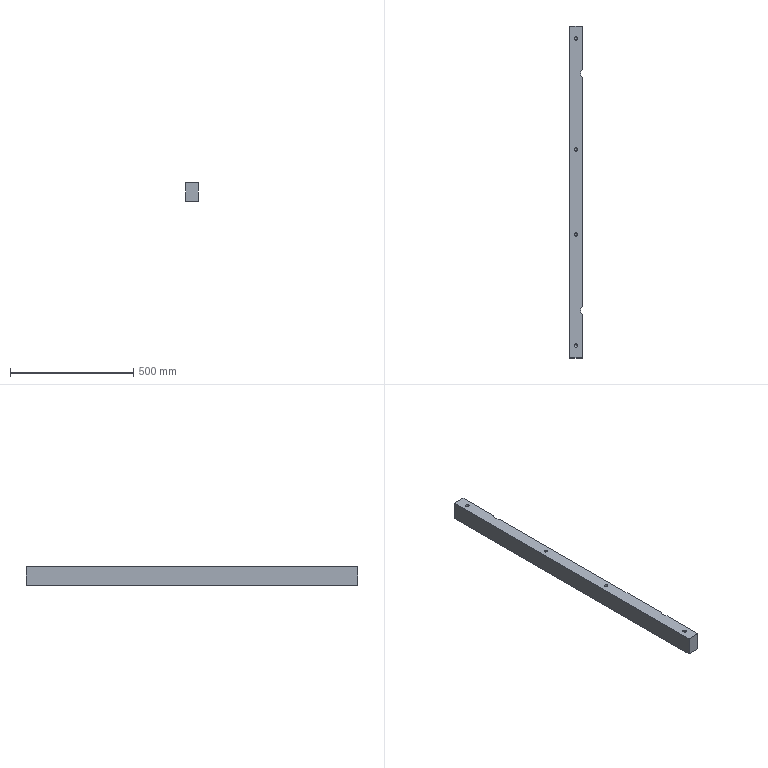Part | NX | features 3 2 | 1 solid | 26 faces | box 50 x 1345 x 75.5 mm | volume 5041133 mm3 | cylinder 10 | plane 8 | cone 8 | commonest cylinder face diameters 14.1 x8 53 x2
STEP:
#1=CARTESIAN_POINT('',(3352.05,-622.5,256.5));
#2=VERTEX_POINT('',#1);
#3=CARTESIAN_POINT('',(3345.,-622.5,256.5));
#4=DIRECTION('',(0.,0.,-1.));
#5=DIRECTION('',(1.,0.,0.));
#6=AXIS2_PLACEMENT_3D('',#3,#4,#5);
#7=CIRCLE('',#6,7.05);
#8=EDGE_CURVE('',#2,#2,#7,.T.);
#9=ORIENTED_EDGE('',*,*,#8,.T.);
#10=EDGE_LOOP('',(#9));
#11=FACE_BOUND('',#10,.T.);
#12=CARTESIAN_POINT('',(3352.05,622.5,256.5));
#13=VERTEX_POINT('',#12);
#14=CARTESIAN_POINT('',(3345.,622.5,256.5));
#15=DIRECTION('',(0.,0.,-1.));
#16=DIRECTION('',(1.,0.,0.));
#17=AXIS2_PLACEMENT_3D('',#14,#15,#16);
#18=CIRCLE('',#17,7.05);
#19=EDGE_CURVE('',#13,#13,#18,.T.);
#20=ORIENTED_EDGE('',*,*,#19,.T.);
#21=EDGE_LOOP('',(#20));
#22=FACE_BOUND('',#21,.T.);
#23=CARTESIAN_POINT('',(3370.,-497.385,256.5));
#24=VERTEX_POINT('',#23);
#25=CARTESIAN_POINT('',(3370.,-462.615,256.5));
#26=VERTEX_POINT('',#25);
#27=CARTESIAN_POINT('',(3390.,-480.,256.5));
#28=DIRECTION('',(0.,0.,-1.));
#29=DIRECTION('',(1.,0.,0.));
#30=AXIS2_PLACEMENT_3D('',#27,#28,#29);
#31=CIRCLE('',#30,26.5);
#32=EDGE_CURVE('',#24,#26,#31,.T.);
#33=ORIENTED_EDGE('',*,*,#32,.T.);
#34=CARTESIAN_POINT('',(3370.,462.615,256.5));
#35=VERTEX_POINT('',#34);
#36=CARTESIAN_POINT('',(3370.,193.,256.5));
#37=DIRECTION('',(0.,1.,0.));
#38=VECTOR('',#37,1000.);
#39=LINE('',#36,#38);
#40=EDGE_CURVE('',#26,#35,#39,.T.);
#41=ORIENTED_EDGE('',*,*,#40,.T.);
#42=CARTESIAN_POINT('',(3370.,497.385,256.5));
#43=VERTEX_POINT('',#42);
#44=CARTESIAN_POINT('',(3390.,480.,256.5));
#45=DIRECTION('',(0.,0.,1.));
#46=DIRECTION('',(1.,0.,0.));
#47=AXIS2_PLACEMENT_3D('',#44,#45,#46);
#48=CIRCLE('',#47,26.5);
#49=EDGE_CURVE('',#43,#35,#48,.T.);
#50=ORIENTED_EDGE('',*,*,#49,.F.);
#51=CARTESIAN_POINT('',(3370.,672.5,256.5));
#52=VERTEX_POINT('',#51);
#53=CARTESIAN_POINT('',(3370.,193.,256.5));
#54=DIRECTION('',(0.,1.,0.));
#55=VECTOR('',#54,1000.);
#56=LINE('',#53,#55);
#57=EDGE_CURVE('',#43,#52,#56,.T.);
#58=ORIENTED_EDGE('',*,*,#57,.T.);
#59=CARTESIAN_POINT('',(3320.,672.5,256.5));
#60=VERTEX_POINT('',#59);
#61=CARTESIAN_POINT('',(1330.,672.5,256.5));
#62=DIRECTION('',(-1.,0.,0.));
#63=VECTOR('',#62,1000.);
#64=LINE('',#61,#63);
#65=EDGE_CURVE('',#52,#60,#64,.T.);
#66=ORIENTED_EDGE('',*,*,#65,.T.);
#67=CARTESIAN_POINT('',(3320.,-672.5,256.5));
#68=VERTEX_POINT('',#67);
#69=CARTESIAN_POINT('',(3320.,193.,256.5));
#70=DIRECTION('',(0.,-1.,0.));
#71=VECTOR('',#70,1000.);
#72=LINE('',#69,#71);
#73=EDGE_CURVE('',#60,#68,#72,.T.);
#74=ORIENTED_EDGE('',*,*,#73,.T.);
#75=CARTESIAN_POINT('',(3370.,-672.5,256.5));
#76=VERTEX_POINT('',#75);
#77=CARTESIAN_POINT('',(1330.,-672.5,256.5));
#78=DIRECTION('',(1.,0.,0.));
#79=VECTOR('',#78,1000.);
#80=LINE('',#77,#79);
#81=EDGE_CURVE('',#68,#76,#80,.T.);
#82=ORIENTED_EDGE('',*,*,#81,.T.);
#83=CARTESIAN_POINT('',(3370.,193.,256.5));
#84=DIRECTION('',(0.,1.,0.));
#85=VECTOR('',#84,1000.);
#86=LINE('',#83,#85);
#87=EDGE_CURVE('',#76,#24,#86,.T.);
#88=ORIENTED_EDGE('',*,*,#87,.T.);
#89=EDGE_LOOP('',(#33,#41,#50,#58,#66,#74,#82,#88));
#90=FACE_BOUND('',#89,.T.);
#91=CARTESIAN_POINT('',(3352.05,172.5,256.5));
#92=VERTEX_POINT('',#91);
#93=CARTESIAN_POINT('',(3345.,172.5,256.5));
#94=DIRECTION('',(0.,0.,-1.));
#95=DIRECTION('',(1.,0.,0.));
#96=AXIS2_PLACEMENT_3D('',#93,#94,#95);
#97=CIRCLE('',#96,7.05);
#98=EDGE_CURVE('',#92,#92,#97,.T.);
#99=ORIENTED_EDGE('',*,*,#98,.T.);
#100=EDGE_LOOP('',(#99));
#101=FACE_BOUND('',#100,.T.);
#102=CARTESIAN_POINT('',(3352.05,-172.5,256.5));
#103=VERTEX_POINT('',#102);
#104=CARTESIAN_POINT('',(3345.,-172.5,256.5));
#105=DIRECTION('',(0.,0.,-1.));
#106=DIRECTION('',(1.,0.,0.));
#107=AXIS2_PLACEMENT_3D('',#104,#105,#106);
#108=CIRCLE('',#107,7.05);
#109=EDGE_CURVE('',#103,#103,#108,.T.);
#110=ORIENTED_EDGE('',*,*,#109,.T.);
#111=EDGE_LOOP('',(#110));
#112=FACE_BOUND('',#111,.T.);
#113=CARTESIAN_POINT('',(1330.,0.,256.5));
#114=DIRECTION('',(0.,0.,1.));
#115=DIRECTION('',(1.,0.,0.));
#116=AXIS2_PLACEMENT_3D('',#113,#114,#115);
#117=PLANE('',#116);
#118=ADVANCED_FACE('',(#11,#22,#90,#101,#112),#117,.T.);
#119=CARTESIAN_POINT('',(3352.05,-172.5,181.));
#120=VERTEX_POINT('',#119);
#121=CARTESIAN_POINT('',(3345.,-172.5,181.));
#122=DIRECTION('',(0.,0.,1.));
#123=DIRECTION('',(1.,0.,0.));
#124=AXIS2_PLACEMENT_3D('',#121,#122,#123);
#125=CIRCLE('',#124,7.05);
#126=EDGE_CURVE('',#120,#120,#125,.T.);
#127=ORIENTED_EDGE('',*,*,#126,.T.);
#128=EDGE_LOOP('',(#127));
#129=FACE_BOUND('',#128,.T.);
#130=CARTESIAN_POINT('',(3352.05,172.5,181.));
#131=VERTEX_POINT('',#130);
#132=CARTESIAN_POINT('',(3345.,172.5,181.));
#133=DIRECTION('',(0.,0.,1.));
#134=DIRECTION('',(1.,0.,0.));
#135=AXIS2_PLACEMENT_3D('',#132,#133,#134);
#136=CIRCLE('',#135,7.05);
#137=EDGE_CURVE('',#131,#131,#136,.T.);
#138=ORIENTED_EDGE('',*,*,#137,.T.);
#139=EDGE_LOOP('',(#138));
#140=FACE_BOUND('',#139,.T.);
#141=CARTESIAN_POINT('',(3370.,-497.385,181.));
#142=VERTEX_POINT('',#141);
#143=CARTESIAN_POINT('',(3370.,-462.615,181.));
#144=VERTEX_POINT('',#143);
#145=CARTESIAN_POINT('',(3390.,-480.,181.));
#146=DIRECTION('',(0.,0.,-1.));
#147=DIRECTION('',(-1.,0.,0.));
#148=AXIS2_PLACEMENT_3D('',#145,#146,#147);
#149=CIRCLE('',#148,26.5);
#150=EDGE_CURVE('',#142,#144,#149,.T.);
#151=ORIENTED_EDGE('',*,*,#150,.F.);
#152=CARTESIAN_POINT('',(3370.,-672.5,181.));
#153=VERTEX_POINT('',#152);
#154=CARTESIAN_POINT('',(3370.,193.,181.));
#155=DIRECTION('',(0.,-1.,0.));
#156=VECTOR('',#155,1000.);
#157=LINE('',#154,#156);
#158=EDGE_CURVE('',#142,#153,#157,.T.);
#159=ORIENTED_EDGE('',*,*,#158,.T.);
#160=CARTESIAN_POINT('',(3320.,-672.5,181.));
#161=VERTEX_POINT('',#160);
#162=CARTESIAN_POINT('',(267.5,-672.5,181.));
#163=DIRECTION('',(1.,0.,0.));
#164=VECTOR('',#163,1000.);
#165=LINE('',#162,#164);
#166=EDGE_CURVE('',#161,#153,#165,.T.);
#167=ORIENTED_EDGE('',*,*,#166,.F.);
#168=CARTESIAN_POINT('',(3320.,672.5,181.));
#169=VERTEX_POINT('',#168);
#170=CARTESIAN_POINT('',(3320.,193.,181.));
#171=DIRECTION('',(0.,1.,0.));
#172=VECTOR('',#171,1000.);
#173=LINE('',#170,#172);
#174=EDGE_CURVE('',#161,#169,#173,.T.);
#175=ORIENTED_EDGE('',*,*,#174,.T.);
#176=CARTESIAN_POINT('',(3370.,672.5,181.));
#177=VERTEX_POINT('',#176);
#178=CARTESIAN_POINT('',(3370.,672.5,181.));
#179=DIRECTION('',(-1.,0.,0.));
#180=VECTOR('',#179,1000.);
#181=LINE('',#178,#180);
#182=EDGE_CURVE('',#177,#169,#181,.T.);
#183=ORIENTED_EDGE('',*,*,#182,.F.);
#184=CARTESIAN_POINT('',(3370.,497.385,181.));
#185=VERTEX_POINT('',#184);
#186=CARTESIAN_POINT('',(3370.,193.,181.));
#187=DIRECTION('',(0.,-1.,0.));
#188=VECTOR('',#187,1000.);
#189=LINE('',#186,#188);
#190=EDGE_CURVE('',#177,#185,#189,.T.);
#191=ORIENTED_EDGE('',*,*,#190,.T.);
#192=CARTESIAN_POINT('',(3370.,462.615,181.));
#193=VERTEX_POINT('',#192);
#194=CARTESIAN_POINT('',(3390.,480.,181.));
#195=DIRECTION('',(0.,0.,1.));
#196=DIRECTION('',(-1.,0.,0.));
#197=AXIS2_PLACEMENT_3D('',#194,#195,#196);
#198=CIRCLE('',#197,26.5);
#199=EDGE_CURVE('',#185,#193,#198,.T.);
#200=ORIENTED_EDGE('',*,*,#199,.T.);
#201=CARTESIAN_POINT('',(3370.,193.,181.));
#202=DIRECTION('',(0.,-1.,0.));
#203=VECTOR('',#202,1000.);
#204=LINE('',#201,#203);
#205=EDGE_CURVE('',#193,#144,#204,.T.);
#206=ORIENTED_EDGE('',*,*,#205,.T.);
#207=EDGE_LOOP('',(#151,#159,#167,#175,#183,#191,#200,#206));
#208=FACE_BOUND('',#207,.T.);
#209=CARTESIAN_POINT('',(3352.05,-622.5,181.));
#210=VERTEX_POINT('',#209);
#211=CARTESIAN_POINT('',(3345.,-622.5,181.));
#212=DIRECTION('',(0.,0.,1.));
#213=DIRECTION('',(1.,0.,0.));
#214=AXIS2_PLACEMENT_3D('',#211,#212,#213);
#215=CIRCLE('',#214,7.05);
#216=EDGE_CURVE('',#210,#210,#215,.T.);
#217=ORIENTED_EDGE('',*,*,#216,.T.);
#218=EDGE_LOOP('',(#217));
#219=FACE_BOUND('',#218,.T.);
#220=CARTESIAN_POINT('',(3352.05,622.5,181.));
#221=VERTEX_POINT('',#220);
#222=CARTESIAN_POINT('',(3345.,622.5,181.));
#223=DIRECTION('',(0.,0.,1.));
#224=DIRECTION('',(1.,0.,0.));
#225=AXIS2_PLACEMENT_3D('',#222,#223,#224);
#226=CIRCLE('',#225,7.05);
#227=EDGE_CURVE('',#221,#221,#226,.T.);
#228=ORIENTED_EDGE('',*,*,#227,.T.);
#229=EDGE_LOOP('',(#228));
#230=FACE_BOUND('',#229,.T.);
#231=CARTESIAN_POINT('',(2100.,193.,181.));
#232=DIRECTION('',(0.,0.,-1.));
#233=DIRECTION('',(1.,0.,0.));
#234=AXIS2_PLACEMENT_3D('',#231,#232,#233);
#235=PLANE('',#234);
#236=ADVANCED_FACE('',(#129,#140,#208,#219,#230),#235,.T.);
#237=CARTESIAN_POINT('',(3370.,-462.615,181.));
#238=DIRECTION('',(0.,0.,1.));
#239=VECTOR('',#238,1000.);
#240=LINE('',#237,#239);
#241=EDGE_CURVE('',#144,#26,#240,.T.);
#242=ORIENTED_EDGE('',*,*,#241,.F.);
#243=ORIENTED_EDGE('',*,*,#205,.F.);
#244=CARTESIAN_POINT('',(3370.,462.615,181.));
#245=DIRECTION('',(0.,0.,1.));
#246=VECTOR('',#245,1000.);
#247=LINE('',#244,#246);
#248=EDGE_CURVE('',#193,#35,#247,.T.);
#249=ORIENTED_EDGE('',*,*,#248,.T.);
#250=ORIENTED_EDGE('',*,*,#40,.F.);
#251=EDGE_LOOP('',(#242,#243,#249,#250));
#252=FACE_BOUND('',#251,.T.);
#253=CARTESIAN_POINT('',(3370.,193.,-1.5));
#254=DIRECTION('',(1.,0.,0.));
#255=DIRECTION('',(0.,0.,-1.));
#256=AXIS2_PLACEMENT_3D('',#253,#254,#255);
#257=PLANE('',#256);
#258=ADVANCED_FACE('',(#252),#257,.T.);
#259=CARTESIAN_POINT('',(3370.,497.385,256.5));
#260=DIRECTION('',(0.,0.,-1.));
#261=VECTOR('',#260,1000.);
#262=LINE('',#259,#261);
#263=EDGE_CURVE('',#43,#185,#262,.T.);
#264=ORIENTED_EDGE('',*,*,#263,.T.);
#265=ORIENTED_EDGE('',*,*,#190,.F.);
#266=CARTESIAN_POINT('',(3370.,672.5,231.5));
#267=DIRECTION('',(0.,0.,-1.));
#268=VECTOR('',#267,1000.);
#269=LINE('',#266,#268);
#270=EDGE_CURVE('',#52,#177,#269,.T.);
#271=ORIENTED_EDGE('',*,*,#270,.F.);
#272=ORIENTED_EDGE('',*,*,#57,.F.);
#273=EDGE_LOOP('',(#264,#265,#271,#272));
#274=FACE_BOUND('',#273,.T.);
#275=CARTESIAN_POINT('',(3370.,193.,-1.5));
#276=DIRECTION('',(1.,0.,0.));
#277=DIRECTION('',(0.,0.,-1.));
#278=AXIS2_PLACEMENT_3D('',#275,#276,#277);
#279=PLANE('',#278);
#280=ADVANCED_FACE('',(#274),#279,.T.);
#281=CARTESIAN_POINT('',(3370.,-497.385,256.5));
#282=DIRECTION('',(0.,0.,-1.));
#283=VECTOR('',#282,1000.);
#284=LINE('',#281,#283);
#285=EDGE_CURVE('',#24,#142,#284,.T.);
#286=ORIENTED_EDGE('',*,*,#285,.F.);
#287=ORIENTED_EDGE('',*,*,#87,.F.);
#288=CARTESIAN_POINT('',(3370.,-672.5,-103.));
#289=DIRECTION('',(0.,0.,1.));
#290=VECTOR('',#289,1000.);
#291=LINE('',#288,#290);
#292=EDGE_CURVE('',#153,#76,#291,.T.);
#293=ORIENTED_EDGE('',*,*,#292,.F.);
#294=ORIENTED_EDGE('',*,*,#158,.F.);
#295=EDGE_LOOP('',(#286,#287,#293,#294));
#296=FACE_BOUND('',#295,.T.);
#297=CARTESIAN_POINT('',(3370.,193.,-1.5));
#298=DIRECTION('',(1.,0.,0.));
#299=DIRECTION('',(0.,0.,-1.));
#300=AXIS2_PLACEMENT_3D('',#297,#298,#299);
#301=PLANE('',#300);
#302=ADVANCED_FACE('',(#296),#301,.T.);
#303=CARTESIAN_POINT('',(3320.,672.5,231.5));
#304=DIRECTION('',(0.,0.,1.));
#305=VECTOR('',#304,1000.);
#306=LINE('',#303,#305);
#307=EDGE_CURVE('',#169,#60,#306,.T.);
#308=ORIENTED_EDGE('',*,*,#307,.F.);
#309=ORIENTED_EDGE('',*,*,#174,.F.);
#310=CARTESIAN_POINT('',(3320.,-672.5,-103.));
#311=DIRECTION('',(0.,0.,-1.));
#312=VECTOR('',#311,1000.);
#313=LINE('',#310,#312);
#314=EDGE_CURVE('',#68,#161,#313,.T.);
#315=ORIENTED_EDGE('',*,*,#314,.F.);
#316=ORIENTED_EDGE('',*,*,#73,.F.);
#317=EDGE_LOOP('',(#308,#309,#315,#316));
#318=FACE_BOUND('',#317,.T.);
#319=CARTESIAN_POINT('',(3320.,193.,-1.5));
#320=DIRECTION('',(-1.,0.,0.));
#321=DIRECTION('',(0.,0.,1.));
#322=AXIS2_PLACEMENT_3D('',#319,#320,#321);
#323=PLANE('',#322);
#324=ADVANCED_FACE('',(#318),#323,.T.);
#325=ORIENTED_EDGE('',*,*,#314,.T.);
#326=ORIENTED_EDGE('',*,*,#166,.T.);
#327=ORIENTED_EDGE('',*,*,#292,.T.);
#328=ORIENTED_EDGE('',*,*,#81,.F.);
#329=EDGE_LOOP('',(#325,#326,#327,#328));
#330=FACE_BOUND('',#329,.T.);
#331=CARTESIAN_POINT('',(267.5,-672.5,-103.));
#332=DIRECTION('',(0.,1.,0.));
#333=DIRECTION('',(1.,0.,0.));
#334=AXIS2_PLACEMENT_3D('',#331,#332,#333);
#335=PLANE('',#334);
#336=ADVANCED_FACE('',(#330),#335,.F.);
#337=ORIENTED_EDGE('',*,*,#270,.T.);
#338=ORIENTED_EDGE('',*,*,#182,.T.);
#339=ORIENTED_EDGE('',*,*,#307,.T.);
#340=ORIENTED_EDGE('',*,*,#65,.F.);
#341=EDGE_LOOP('',(#337,#338,#339,#340));
#342=FACE_BOUND('',#341,.T.);
#343=CARTESIAN_POINT('',(3370.,672.5,231.5));
#344=DIRECTION('',(0.,1.,0.));
#345=DIRECTION('',(0.,0.,-1.));
#346=AXIS2_PLACEMENT_3D('',#343,#344,#345);
#347=PLANE('',#346);
#348=ADVANCED_FACE('',(#342),#347,.T.);
#349=ORIENTED_EDGE('',*,*,#49,.T.);
#350=ORIENTED_EDGE('',*,*,#248,.F.);
#351=ORIENTED_EDGE('',*,*,#199,.F.);
#352=ORIENTED_EDGE('',*,*,#263,.F.);
#353=EDGE_LOOP('',(#349,#350,#351,#352));
#354=FACE_BOUND('',#353,.T.);
#355=CARTESIAN_POINT('',(3390.,480.,-181.));
#356=DIRECTION('',(0.,0.,1.));
#357=DIRECTION('',(-1.,0.,0.));
#358=AXIS2_PLACEMENT_3D('',#355,#356,#357);
#359=CYLINDRICAL_SURFACE('',#358,26.5);
#360=ADVANCED_FACE('',(#354),#359,.F.);
#361=ORIENTED_EDGE('',*,*,#32,.F.);
#362=ORIENTED_EDGE('',*,*,#285,.T.);
#363=ORIENTED_EDGE('',*,*,#150,.T.);
#364=ORIENTED_EDGE('',*,*,#241,.T.);
#365=EDGE_LOOP('',(#361,#362,#363,#364));
#366=FACE_BOUND('',#365,.T.);
#367=CARTESIAN_POINT('',(3390.,-480.,-181.));
#368=DIRECTION('',(0.,0.,1.));
#369=DIRECTION('',(-1.,0.,0.));
#370=AXIS2_PLACEMENT_3D('',#367,#368,#369);
#371=CYLINDRICAL_SURFACE('',#370,26.5);
#372=ADVANCED_FACE('',(#366),#371,.F.);
#373=CARTESIAN_POINT('',(3352.05,172.5,188.95));
#374=VERTEX_POINT('',#373);
#375=CARTESIAN_POINT('',(3345.,172.5,188.95));
#376=DIRECTION('',(0.,0.,1.));
#377=DIRECTION('',(1.,0.,0.));
#378=AXIS2_PLACEMENT_3D('',#375,#376,#377);
#379=CIRCLE('',#378,7.05);
#380=EDGE_CURVE('',#374,#374,#379,.T.);
#381=ORIENTED_EDGE('',*,*,#380,.T.);
#382=EDGE_LOOP('',(#381));
#383=FACE_BOUND('',#382,.T.);
#384=ORIENTED_EDGE('',*,*,#137,.F.);
#385=EDGE_LOOP('',(#384));
#386=FACE_BOUND('',#385,.T.);
#387=CARTESIAN_POINT('',(3345.,172.5,181.));
#388=DIRECTION('',(0.,0.,1.));
#389=DIRECTION('',(-1.,0.,0.));
#390=AXIS2_PLACEMENT_3D('',#387,#388,#389);
#391=CYLINDRICAL_SURFACE('',#390,7.05);
#392=ADVANCED_FACE('',(#383,#386),#391,.F.);
#393=CARTESIAN_POINT('',(3345.,172.5,196.));
#394=VERTEX_POINT('',#393);
#395=VERTEX_LOOP('',#394);
#396=FACE_BOUND('',#395,.T.);
#397=ORIENTED_EDGE('',*,*,#380,.F.);
#398=EDGE_LOOP('',(#397));
#399=FACE_BOUND('',#398,.T.);
#400=CARTESIAN_POINT('',(3345.,172.5,188.95));
#401=DIRECTION('',(0.,0.,-1.));
#402=DIRECTION('',(1.,0.,0.));
#403=AXIS2_PLACEMENT_3D('',#400,#401,#402);
#404=CONICAL_SURFACE('',#403,7.05,0.7854);
#405=ADVANCED_FACE('',(#396,#399),#404,.F.);
#406=CARTESIAN_POINT('',(3352.05,-622.5,188.95));
#407=VERTEX_POINT('',#406);
#408=CARTESIAN_POINT('',(3345.,-622.5,188.95));
#409=DIRECTION('',(0.,0.,1.));
#410=DIRECTION('',(1.,0.,0.));
#411=AXIS2_PLACEMENT_3D('',#408,#409,#410);
#412=CIRCLE('',#411,7.05);
#413=EDGE_CURVE('',#407,#407,#412,.T.);
#414=ORIENTED_EDGE('',*,*,#413,.T.);
#415=EDGE_LOOP('',(#414));
#416=FACE_BOUND('',#415,.T.);
#417=ORIENTED_EDGE('',*,*,#216,.F.);
#418=EDGE_LOOP('',(#417));
#419=FACE_BOUND('',#418,.T.);
#420=CARTESIAN_POINT('',(3345.,-622.5,181.));
#421=DIRECTION('',(0.,0.,1.));
#422=DIRECTION('',(-1.,0.,0.));
#423=AXIS2_PLACEMENT_3D('',#420,#421,#422);
#424=CYLINDRICAL_SURFACE('',#423,7.05);
#425=ADVANCED_FACE('',(#416,#419),#424,.F.);
#426=CARTESIAN_POINT('',(3345.,-622.5,196.));
#427=VERTEX_POINT('',#426);
#428=VERTEX_LOOP('',#427);
#429=FACE_BOUND('',#428,.T.);
#430=ORIENTED_EDGE('',*,*,#413,.F.);
#431=EDGE_LOOP('',(#430));
#432=FACE_BOUND('',#431,.T.);
#433=CARTESIAN_POINT('',(3345.,-622.5,188.95));
#434=DIRECTION('',(0.,0.,-1.));
#435=DIRECTION('',(1.,0.,0.));
#436=AXIS2_PLACEMENT_3D('',#433,#434,#435);
#437=CONICAL_SURFACE('',#436,7.05,0.7854);
#438=ADVANCED_FACE('',(#429,#432),#437,.F.);
#439=CARTESIAN_POINT('',(3352.05,-172.5,188.95));
#440=VERTEX_POINT('',#439);
#441=CARTESIAN_POINT('',(3345.,-172.5,188.95));
#442=DIRECTION('',(0.,0.,1.));
#443=DIRECTION('',(1.,0.,0.));
#444=AXIS2_PLACEMENT_3D('',#441,#442,#443);
#445=CIRCLE('',#444,7.05);
#446=EDGE_CURVE('',#440,#440,#445,.T.);
#447=ORIENTED_EDGE('',*,*,#446,.T.);
#448=EDGE_LOOP('',(#447));
#449=FACE_BOUND('',#448,.T.);
#450=ORIENTED_EDGE('',*,*,#126,.F.);
#451=EDGE_LOOP('',(#450));
#452=FACE_BOUND('',#451,.T.);
#453=CARTESIAN_POINT('',(3345.,-172.5,181.));
#454=DIRECTION('',(0.,0.,1.));
#455=DIRECTION('',(-1.,0.,0.));
#456=AXIS2_PLACEMENT_3D('',#453,#454,#455);
#457=CYLINDRICAL_SURFACE('',#456,7.05);
#458=ADVANCED_FACE('',(#449,#452),#457,.F.);
#459=CARTESIAN_POINT('',(3345.,-172.5,196.));
#460=VERTEX_POINT('',#459);
#461=VERTEX_LOOP('',#460);
#462=FACE_BOUND('',#461,.T.);
#463=ORIENTED_EDGE('',*,*,#446,.F.);
#464=EDGE_LOOP('',(#463));
#465=FACE_BOUND('',#464,.T.);
#466=CARTESIAN_POINT('',(3345.,-172.5,188.95));
#467=DIRECTION('',(0.,0.,-1.));
#468=DIRECTION('',(1.,0.,0.));
#469=AXIS2_PLACEMENT_3D('',#466,#467,#468);
#470=CONICAL_SURFACE('',#469,7.05,0.7854);
#471=ADVANCED_FACE('',(#462,#465),#470,.F.);
#472=CARTESIAN_POINT('',(3352.05,622.5,188.95));
#473=VERTEX_POINT('',#472);
#474=CARTESIAN_POINT('',(3345.,622.5,188.95));
#475=DIRECTION('',(0.,0.,1.));
#476=DIRECTION('',(1.,0.,0.));
#477=AXIS2_PLACEMENT_3D('',#474,#475,#476);
#478=CIRCLE('',#477,7.05);
#479=EDGE_CURVE('',#473,#473,#478,.T.);
#480=ORIENTED_EDGE('',*,*,#479,.T.);
#481=EDGE_LOOP('',(#480));
#482=FACE_BOUND('',#481,.T.);
#483=ORIENTED_EDGE('',*,*,#227,.F.);
#484=EDGE_LOOP('',(#483));
#485=FACE_BOUND('',#484,.T.);
#486=CARTESIAN_POINT('',(3345.,622.5,181.));
#487=DIRECTION('',(0.,0.,1.));
#488=DIRECTION('',(-1.,0.,0.));
#489=AXIS2_PLACEMENT_3D('',#486,#487,#488);
#490=CYLINDRICAL_SURFACE('',#489,7.05);
#491=ADVANCED_FACE('',(#482,#485),#490,.F.);
#492=CARTESIAN_POINT('',(3345.,622.5,196.));
#493=VERTEX_POINT('',#492);
#494=VERTEX_LOOP('',#493);
#495=FACE_BOUND('',#494,.T.);
#496=ORIENTED_EDGE('',*,*,#479,.F.);
#497=EDGE_LOOP('',(#496));
#498=FACE_BOUND('',#497,.T.);
#499=CARTESIAN_POINT('',(3345.,622.5,188.95));
#500=DIRECTION('',(0.,0.,-1.));
#501=DIRECTION('',(1.,0.,0.));
#502=AXIS2_PLACEMENT_3D('',#499,#500,#501);
#503=CONICAL_SURFACE('',#502,7.05,0.7854);
#504=ADVANCED_FACE('',(#495,#498),#503,.F.);
#505=CARTESIAN_POINT('',(3337.95,622.5,248.55));
#506=VERTEX_POINT('',#505);
#507=CARTESIAN_POINT('',(3345.,622.5,248.55));
#508=DIRECTION('',(0.,0.,-1.));
#509=DIRECTION('',(-1.,0.,0.));
#510=AXIS2_PLACEMENT_3D('',#507,#508,#509);
#511=CIRCLE('',#510,7.05);
#512=EDGE_CURVE('',#506,#506,#511,.T.);
#513=ORIENTED_EDGE('',*,*,#512,.T.);
#514=EDGE_LOOP('',(#513));
#515=FACE_BOUND('',#514,.T.);
#516=ORIENTED_EDGE('',*,*,#19,.F.);
#517=EDGE_LOOP('',(#516));
#518=FACE_BOUND('',#517,.T.);
#519=CARTESIAN_POINT('',(3345.,622.5,256.5));
#520=DIRECTION('',(0.,0.,-1.));
#521=DIRECTION('',(-1.,0.,0.));
#522=AXIS2_PLACEMENT_3D('',#519,#520,#521);
#523=CYLINDRICAL_SURFACE('',#522,7.05);
#524=ADVANCED_FACE('',(#515,#518),#523,.F.);
#525=CARTESIAN_POINT('',(3345.,622.5,241.5));
#526=VERTEX_POINT('',#525);
#527=VERTEX_LOOP('',#526);
#528=FACE_BOUND('',#527,.T.);
#529=ORIENTED_EDGE('',*,*,#512,.F.);
#530=EDGE_LOOP('',(#529));
#531=FACE_BOUND('',#530,.T.);
#532=CARTESIAN_POINT('',(3345.,622.5,248.55));
#533=DIRECTION('',(0.,0.,1.));
#534=DIRECTION('',(-1.,0.,0.));
#535=AXIS2_PLACEMENT_3D('',#532,#533,#534);
#536=CONICAL_SURFACE('',#535,7.05,0.7854);
#537=ADVANCED_FACE('',(#528,#531),#536,.F.);
#538=CARTESIAN_POINT('',(3337.95,172.5,248.55));
#539=VERTEX_POINT('',#538);
#540=CARTESIAN_POINT('',(3345.,172.5,248.55));
#541=DIRECTION('',(0.,0.,-1.));
#542=DIRECTION('',(-1.,0.,0.));
#543=AXIS2_PLACEMENT_3D('',#540,#541,#542);
#544=CIRCLE('',#543,7.05);
#545=EDGE_CURVE('',#539,#539,#544,.T.);
#546=ORIENTED_EDGE('',*,*,#545,.T.);
#547=EDGE_LOOP('',(#546));
#548=FACE_BOUND('',#547,.T.);
#549=ORIENTED_EDGE('',*,*,#98,.F.);
#550=EDGE_LOOP('',(#549));
#551=FACE_BOUND('',#550,.T.);
#552=CARTESIAN_POINT('',(3345.,172.5,256.5));
#553=DIRECTION('',(0.,0.,-1.));
#554=DIRECTION('',(-1.,0.,0.));
#555=AXIS2_PLACEMENT_3D('',#552,#553,#554);
#556=CYLINDRICAL_SURFACE('',#555,7.05);
#557=ADVANCED_FACE('',(#548,#551),#556,.F.);
#558=CARTESIAN_POINT('',(3345.,172.5,241.5));
#559=VERTEX_POINT('',#558);
#560=VERTEX_LOOP('',#559);
#561=FACE_BOUND('',#560,.T.);
#562=ORIENTED_EDGE('',*,*,#545,.F.);
#563=EDGE_LOOP('',(#562));
#564=FACE_BOUND('',#563,.T.);
#565=CARTESIAN_POINT('',(3345.,172.5,248.55));
#566=DIRECTION('',(0.,0.,1.));
#567=DIRECTION('',(-1.,0.,0.));
#568=AXIS2_PLACEMENT_3D('',#565,#566,#567);
#569=CONICAL_SURFACE('',#568,7.05,0.7854);
#570=ADVANCED_FACE('',(#561,#564),#569,.F.);
#571=CARTESIAN_POINT('',(3337.95,-622.5,248.55));
#572=VERTEX_POINT('',#571);
#573=CARTESIAN_POINT('',(3345.,-622.5,248.55));
#574=DIRECTION('',(0.,0.,-1.));
#575=DIRECTION('',(-1.,0.,0.));
#576=AXIS2_PLACEMENT_3D('',#573,#574,#575);
#577=CIRCLE('',#576,7.05);
#578=EDGE_CURVE('',#572,#572,#577,.T.);
#579=ORIENTED_EDGE('',*,*,#578,.T.);
#580=EDGE_LOOP('',(#579));
#581=FACE_BOUND('',#580,.T.);
#582=ORIENTED_EDGE('',*,*,#8,.F.);
#583=EDGE_LOOP('',(#582));
#584=FACE_BOUND('',#583,.T.);
#585=CARTESIAN_POINT('',(3345.,-622.5,256.5));
#586=DIRECTION('',(0.,0.,-1.));
#587=DIRECTION('',(-1.,0.,0.));
#588=AXIS2_PLACEMENT_3D('',#585,#586,#587);
#589=CYLINDRICAL_SURFACE('',#588,7.05);
#590=ADVANCED_FACE('',(#581,#584),#589,.F.);
#591=CARTESIAN_POINT('',(3345.,-622.5,241.5));
#592=VERTEX_POINT('',#591);
#593=VERTEX_LOOP('',#592);
#594=FACE_BOUND('',#593,.T.);
#595=ORIENTED_EDGE('',*,*,#578,.F.);
#596=EDGE_LOOP('',(#595));
#597=FACE_BOUND('',#596,.T.);
#598=CARTESIAN_POINT('',(3345.,-622.5,248.55));
#599=DIRECTION('',(0.,0.,1.));
#600=DIRECTION('',(-1.,0.,0.));
#601=AXIS2_PLACEMENT_3D('',#598,#599,#600);
#602=CONICAL_SURFACE('',#601,7.05,0.7854);
#603=ADVANCED_FACE('',(#594,#597),#602,.F.);
#604=CARTESIAN_POINT('',(3337.95,-172.5,248.55));
#605=VERTEX_POINT('',#604);
#606=CARTESIAN_POINT('',(3345.,-172.5,248.55));
#607=DIRECTION('',(0.,0.,-1.));
#608=DIRECTION('',(-1.,0.,0.));
#609=AXIS2_PLACEMENT_3D('',#606,#607,#608);
#610=CIRCLE('',#609,7.05);
#611=EDGE_CURVE('',#605,#605,#610,.T.);
#612=ORIENTED_EDGE('',*,*,#611,.T.);
#613=EDGE_LOOP('',(#612));
#614=FACE_BOUND('',#613,.T.);
#615=ORIENTED_EDGE('',*,*,#109,.F.);
#616=EDGE_LOOP('',(#615));
#617=FACE_BOUND('',#616,.T.);
#618=CARTESIAN_POINT('',(3345.,-172.5,256.5));
#619=DIRECTION('',(0.,0.,-1.));
#620=DIRECTION('',(-1.,0.,0.));
#621=AXIS2_PLACEMENT_3D('',#618,#619,#620);
#622=CYLINDRICAL_SURFACE('',#621,7.05);
#623=ADVANCED_FACE('',(#614,#617),#622,.F.);
#624=CARTESIAN_POINT('',(3345.,-172.5,241.5));
#625=VERTEX_POINT('',#624);
#626=VERTEX_LOOP('',#625);
#627=FACE_BOUND('',#626,.T.);
#628=ORIENTED_EDGE('',*,*,#611,.F.);
#629=EDGE_LOOP('',(#628));
#630=FACE_BOUND('',#629,.T.);
#631=CARTESIAN_POINT('',(3345.,-172.5,248.55));
#632=DIRECTION('',(0.,0.,1.));
#633=DIRECTION('',(-1.,0.,0.));
#634=AXIS2_PLACEMENT_3D('',#631,#632,#633);
#635=CONICAL_SURFACE('',#634,7.05,0.7854);
#636=ADVANCED_FACE('',(#627,#630),#635,.F.);
#637=CLOSED_SHELL('',(#118,#236,#258,#280,#302,#324,#336,#348,#360,#372,#392,#405,#425,#438,#458,#471,#491,#504,#524,#537,#557,#570,#590,#603,#623,#636));
#638=MANIFOLD_SOLID_BREP('',#637);
#639=(LENGTH_UNIT()NAMED_UNIT(*)SI_UNIT(.MILLI.,.METRE.));
#640=UNCERTAINTY_MEASURE_WITH_UNIT(LENGTH_MEASURE(0.00001),#639,'','');
#641=(NAMED_UNIT(*)PLANE_ANGLE_UNIT()SI_UNIT($,.RADIAN.));
#642=(NAMED_UNIT(*)SI_UNIT($,.STERADIAN.)SOLID_ANGLE_UNIT());
#643=(GEOMETRIC_REPRESENTATION_CONTEXT(3)GLOBAL_UNCERTAINTY_ASSIGNED_CONTEXT((#640))GLOBAL_UNIT_ASSIGNED_CONTEXT((#639,#641,#642))REPRESENTATION_CONTEXT('',''));
#644=ADVANCED_BREP_SHAPE_REPRESENTATION('',(#638),#643);